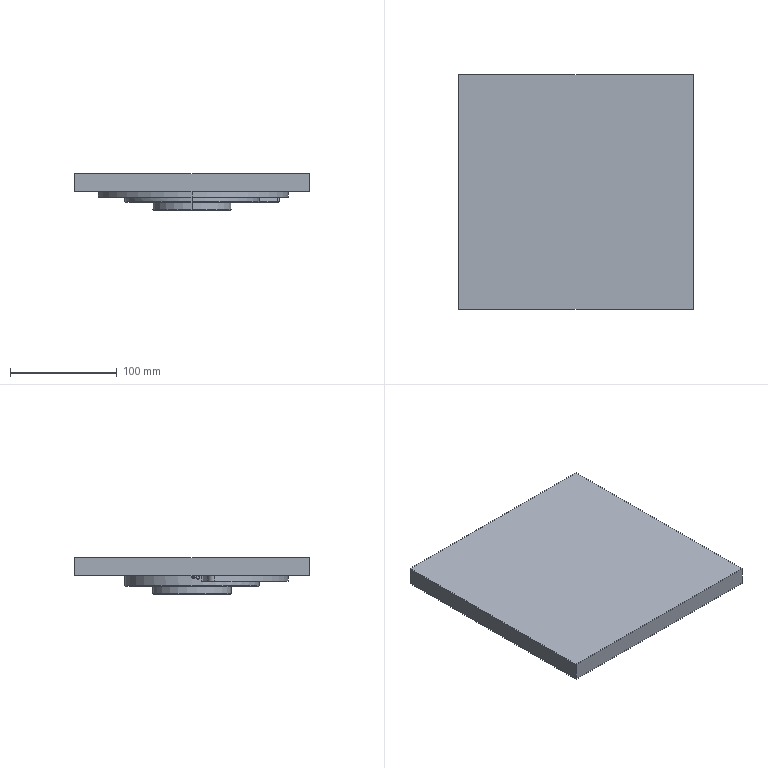NC program | NX | posted with a generic post | part box 220 x 220 x 34.5 mm
Lines 1 to 74 of 14163:
N10 G17 G21 G94 G90
(DRILLING_COPY_1 , TOOL : D6A45)
N12 T18 M6
N14 G54
N16 G17 G0 G90 X47. Y46. S3000 M3
N18 G43 Z30. H18
N20 G94 G81 G98 Z-1.55 F200. R3.
N22 Y36.
N24 G80
N26 G0 X47. Y36. Z30.
(DRILLING_COPY_1_COPY , TOOL : D6A45)
N28 X71.857 Y29.032
N30 G81 Z-2.6 F200. R3.
N32 X36. Y38.5
N34 X35.184 Y69.053
N36 X-22.659 Y74.114
N38 X-56.68 Y52.855
N40 X-75.514 Y17.434
N42 X-74.114 Y-22.659
N44 G80
N46 G0 X-74.114 Y-22.659 Z30.
N48 M5
(DRILLING_COPY_1_COPY_1 , TOOL : 2.6ZT)
N50 T12 M6
N52 G54
N54 G17 G0 G90 X47. Y46. S3000 M3
N56 G43 Z30. H12
N58 G94 G83 G98 Z-8.251 F120. Q2. R3.
N60 Y36.
N62 G80
N64 G0 X47. Y36. Z30.
N66 M5
(DRILLING_COPY_1_COPY_1_COPY_1 , TOOL : 5.2ZT)
N68 T15 M6
N70 G54
N72 G17 G0 G90 X-74.114 Y-22.659 S3000 M3
N74 G43 Z30. H15
N76 G94 G83 G98 Z-15.002 F300. Q2. R3.
N78 X-75.514 Y17.434
N80 X-56.68 Y52.855
N82 X-22.659 Y74.114
N84 X35.184 Y69.053
N86 X71.857 Y29.032
N88 G80
N90 G0 X71.857 Y29.032 Z30.
(DRILLING_COPY_1_COPY_1_COPY_1_COPY_2 , TOOL : 5.2ZT)
N92 X36. Y38.5
N94 G83 Z-20.002 F300. Q2. R3.
N96 G80
N98 G0 X36. Y38.5 Z30.
N100 M5
(DRILLING_COPY_1_COPY_1_COPY_1_COPY_1 , TOOL : 4.5ZT)
N102 T14 M6
N104 G54
N106 G17 G0 G90 X-36.641 Y-37.599 S3000 M3
N108 G43 Z30. H14
N110 G94 G83 G98 Z-19.852 F300. Q2. R-7.
N112 G80
N114 G0 X-36.641 Y-37.599 Z30.
N116 M5